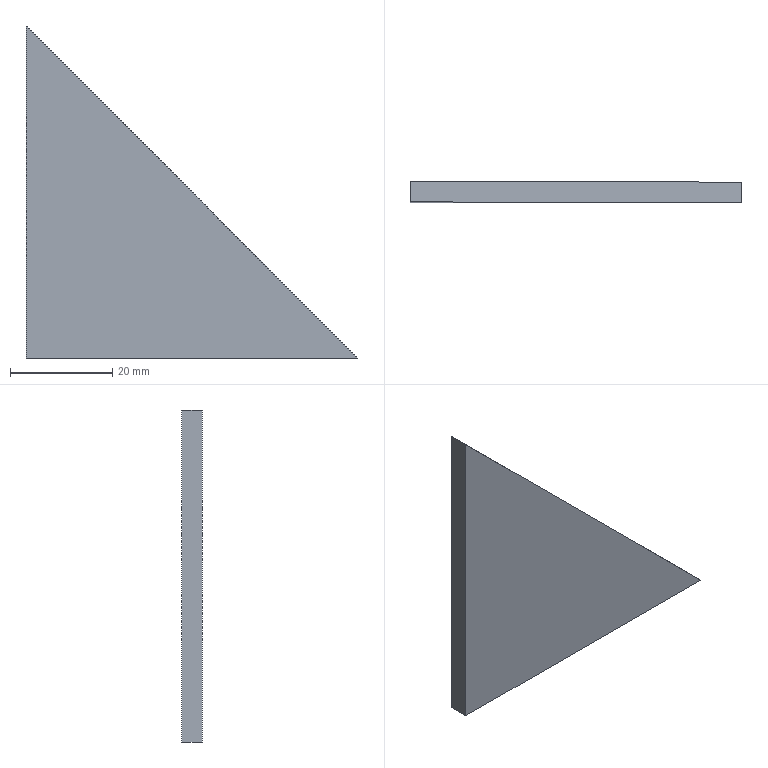Part | SolidWorks | features BaseBody 1 | 1 solid | 5 faces | box 65 x 4 x 65 mm | volume 8450 mm3 | plane 5
STEP:
#1=CARTESIAN_POINT('',(65.,0.,0.));
#2=VERTEX_POINT('',#1);
#3=CARTESIAN_POINT('',(0.,0.,65.));
#4=VERTEX_POINT('',#3);
#5=CARTESIAN_POINT('',(65.,0.,0.));
#6=DIRECTION('',(-0.7071,0.,0.7071));
#7=VECTOR('',#6,1000.);
#8=LINE('',#5,#7);
#9=EDGE_CURVE('',#2,#4,#8,.T.);
#10=ORIENTED_EDGE('',*,*,#9,.F.);
#11=CARTESIAN_POINT('',(0.,0.,0.));
#12=VERTEX_POINT('',#11);
#13=CARTESIAN_POINT('',(22.981,0.,0.));
#14=DIRECTION('',(1.,0.,0.));
#15=VECTOR('',#14,1000.);
#16=LINE('',#13,#15);
#17=EDGE_CURVE('',#12,#2,#16,.T.);
#18=ORIENTED_EDGE('',*,*,#17,.F.);
#19=CARTESIAN_POINT('',(0.,0.,22.981));
#20=DIRECTION('',(0.,0.,-1.));
#21=VECTOR('',#20,1000.);
#22=LINE('',#19,#21);
#23=EDGE_CURVE('',#4,#12,#22,.T.);
#24=ORIENTED_EDGE('',*,*,#23,.F.);
#25=EDGE_LOOP('',(#10,#18,#24));
#26=FACE_OUTER_BOUND('',#25,.T.);
#27=CARTESIAN_POINT('',(22.981,0.,22.981));
#28=DIRECTION('',(0.,-1.,0.));
#29=DIRECTION('',(0.,0.,-1.));
#30=AXIS2_PLACEMENT_3D('',#27,#28,#29);
#31=PLANE('',#30);
#32=ADVANCED_FACE('',(#26),#31,.F.);
#33=CARTESIAN_POINT('',(0.,-4.,0.));
#34=VERTEX_POINT('',#33);
#35=CARTESIAN_POINT('',(0.,0.,0.));
#36=DIRECTION('',(0.,1.,0.));
#37=VECTOR('',#36,1000.);
#38=LINE('',#35,#37);
#39=EDGE_CURVE('',#34,#12,#38,.T.);
#40=ORIENTED_EDGE('',*,*,#39,.F.);
#41=CARTESIAN_POINT('',(0.,-4.,65.));
#42=VERTEX_POINT('',#41);
#43=CARTESIAN_POINT('',(0.,-4.,65.));
#44=DIRECTION('',(0.,0.,-1.));
#45=VECTOR('',#44,1000.);
#46=LINE('',#43,#45);
#47=EDGE_CURVE('',#42,#34,#46,.T.);
#48=ORIENTED_EDGE('',*,*,#47,.F.);
#49=CARTESIAN_POINT('',(0.,0.,65.));
#50=DIRECTION('',(0.,-1.,0.));
#51=VECTOR('',#50,1000.);
#52=LINE('',#49,#51);
#53=EDGE_CURVE('',#4,#42,#52,.T.);
#54=ORIENTED_EDGE('',*,*,#53,.F.);
#55=ORIENTED_EDGE('',*,*,#23,.T.);
#56=EDGE_LOOP('',(#40,#48,#54,#55));
#57=FACE_OUTER_BOUND('',#56,.T.);
#58=CARTESIAN_POINT('',(0.,0.,65.));
#59=DIRECTION('',(1.,0.,0.));
#60=DIRECTION('',(0.,0.,-1.));
#61=AXIS2_PLACEMENT_3D('',#58,#59,#60);
#62=PLANE('',#61);
#63=ADVANCED_FACE('',(#57),#62,.F.);
#64=ORIENTED_EDGE('',*,*,#53,.T.);
#65=CARTESIAN_POINT('',(65.,-4.,0.));
#66=VERTEX_POINT('',#65);
#67=CARTESIAN_POINT('',(65.,-4.,0.));
#68=DIRECTION('',(-0.7071,0.,0.7071));
#69=VECTOR('',#68,1000.);
#70=LINE('',#67,#69);
#71=EDGE_CURVE('',#66,#42,#70,.T.);
#72=ORIENTED_EDGE('',*,*,#71,.F.);
#73=CARTESIAN_POINT('',(65.,0.,0.));
#74=DIRECTION('',(0.,-1.,0.));
#75=VECTOR('',#74,1000.);
#76=LINE('',#73,#75);
#77=EDGE_CURVE('',#2,#66,#76,.T.);
#78=ORIENTED_EDGE('',*,*,#77,.F.);
#79=ORIENTED_EDGE('',*,*,#9,.T.);
#80=EDGE_LOOP('',(#64,#72,#78,#79));
#81=FACE_OUTER_BOUND('',#80,.T.);
#82=CARTESIAN_POINT('',(65.,0.,0.));
#83=DIRECTION('',(-0.7071,0.,-0.7071));
#84=DIRECTION('',(-0.7071,0.,0.7071));
#85=AXIS2_PLACEMENT_3D('',#82,#83,#84);
#86=PLANE('',#85);
#87=ADVANCED_FACE('',(#81),#86,.F.);
#88=ORIENTED_EDGE('',*,*,#77,.T.);
#89=CARTESIAN_POINT('',(0.,-4.,0.));
#90=DIRECTION('',(1.,0.,0.));
#91=VECTOR('',#90,1000.);
#92=LINE('',#89,#91);
#93=EDGE_CURVE('',#34,#66,#92,.T.);
#94=ORIENTED_EDGE('',*,*,#93,.F.);
#95=ORIENTED_EDGE('',*,*,#39,.T.);
#96=ORIENTED_EDGE('',*,*,#17,.T.);
#97=EDGE_LOOP('',(#88,#94,#95,#96));
#98=FACE_OUTER_BOUND('',#97,.T.);
#99=CARTESIAN_POINT('',(0.,0.,0.));
#100=DIRECTION('',(0.,0.,1.));
#101=DIRECTION('',(1.,0.,0.));
#102=AXIS2_PLACEMENT_3D('',#99,#100,#101);
#103=PLANE('',#102);
#104=ADVANCED_FACE('',(#98),#103,.F.);
#105=ORIENTED_EDGE('',*,*,#71,.T.);
#106=ORIENTED_EDGE('',*,*,#47,.T.);
#107=ORIENTED_EDGE('',*,*,#93,.T.);
#108=EDGE_LOOP('',(#105,#106,#107));
#109=FACE_OUTER_BOUND('',#108,.T.);
#110=CARTESIAN_POINT('',(22.981,-4.,22.981));
#111=DIRECTION('',(0.,-1.,0.));
#112=DIRECTION('',(0.,0.,-1.));
#113=AXIS2_PLACEMENT_3D('',#110,#111,#112);
#114=PLANE('',#113);
#115=ADVANCED_FACE('',(#109),#114,.T.);
#116=CLOSED_SHELL('',(#32,#63,#87,#104,#115));
#117=MANIFOLD_SOLID_BREP('',#116);
#118=CARTESIAN_POINT('',(0.,0.,0.));
#119=DIRECTION('',(0.,0.,1.));
#120=DIRECTION('',(1.,0.,0.));
#121=AXIS2_PLACEMENT_3D('',#118,#119,#120);
#122=(LENGTH_UNIT()NAMED_UNIT(*)SI_UNIT(.MILLI.,.METRE.));
#123=UNCERTAINTY_MEASURE_WITH_UNIT(LENGTH_MEASURE(0.00001),#122,'','');
#124=(NAMED_UNIT(*)PLANE_ANGLE_UNIT()SI_UNIT($,.RADIAN.));
#125=(NAMED_UNIT(*)SI_UNIT($,.STERADIAN.)SOLID_ANGLE_UNIT());
#126=(GEOMETRIC_REPRESENTATION_CONTEXT(3)GLOBAL_UNCERTAINTY_ASSIGNED_CONTEXT((#123))GLOBAL_UNIT_ASSIGNED_CONTEXT((#122,#124,#125))REPRESENTATION_CONTEXT('',''));
#127=ADVANCED_BREP_SHAPE_REPRESENTATION('',(#117,#121),#126);